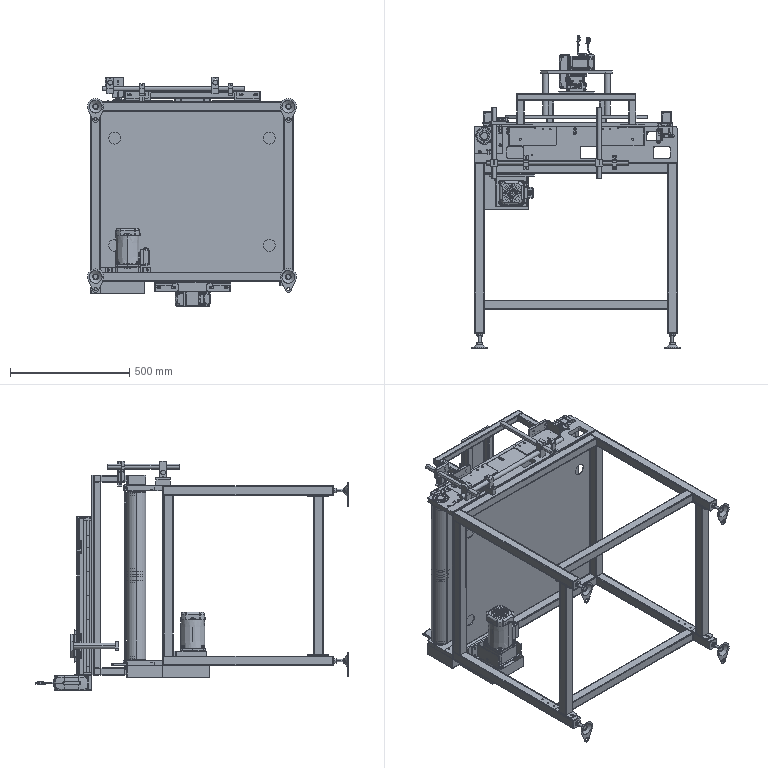Part | SolidWorks | features ReferencePattern 2, CompositeCurve 1, MirrorCompFeat 1 | 165 solids | 7315 faces | volume 25748774 mm3 | cylinder 3063 | plane 2850 | spline 930 | cone 423 | sphere 26 | torus 23 | commonest cylinder face diameters 5 x230 6 x194 4 x179 1 x145 8 x144 2 x128